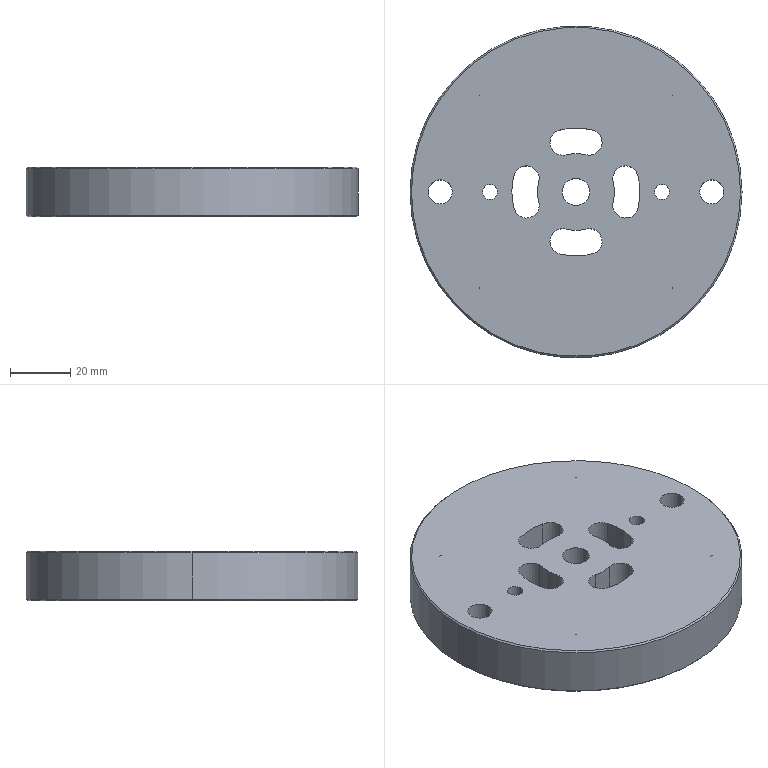Part | STEP file | 11-FG-Z00911 | 1 solid | 59 faces | box 110 x 110 x 16.5 mm | volume 142443 mm3 | cylinder 44 | cone 12 | plane 3 | commonest cylinder face diameters 5 x12 8.5 x12 25.5 x5 42.474 x5 8 x4 9 x2